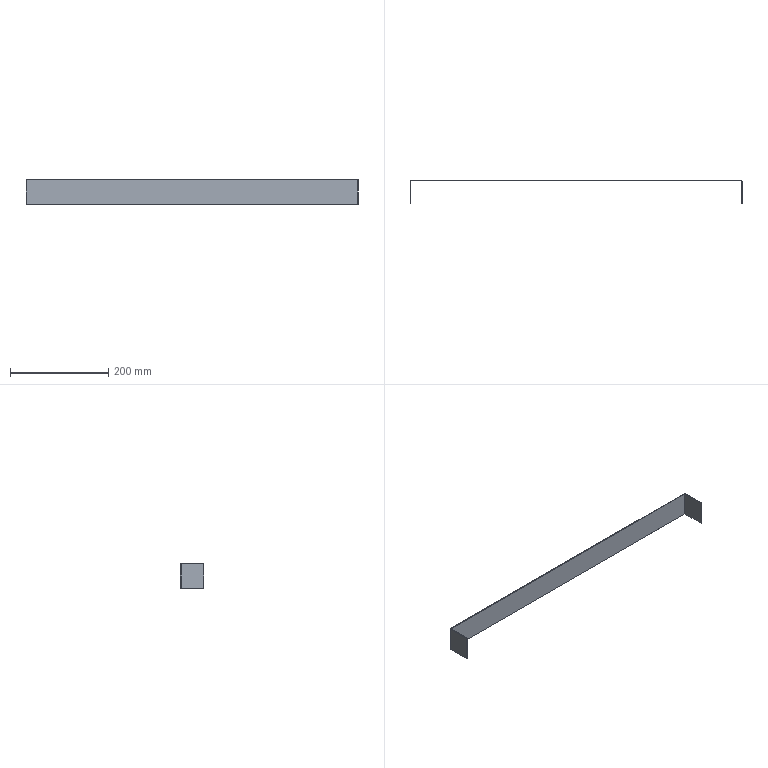Part | STEP file | C4 connector | 1 solid | 14 faces | box 677 x 48.5 x 50 mm | volume 57745 mm3 | plane 10 | cylinder 4 | commonest cylinder face diameters 1 x2 4 x2
STEP:
#1=CARTESIAN_POINT('',(0.,0.,0.));
#2=DIRECTION('',(0.,0.,1.));
#3=DIRECTION('',(1.,0.,0.));
#4=AXIS2_PLACEMENT_3D('',#1,#2,#3);
#5=CARTESIAN_POINT('',(3.5,48.5,0.));
#6=VERTEX_POINT('',#5);
#7=CARTESIAN_POINT('',(1.5,46.5,0.));
#8=VERTEX_POINT('',#7);
#9=CARTESIAN_POINT('',(3.5,46.5,0.));
#10=DIRECTION('',(0.,0.,1.));
#11=DIRECTION('',(0.,1.,0.));
#12=AXIS2_PLACEMENT_3D('',#9,#10,#11);
#13=CIRCLE('',#12,2.);
#14=CARTESIAN_POINT('',(3.5,46.5,0.));
#15=DIRECTION('',(0.,0.,1.));
#16=DIRECTION('',(0.,1.,0.));
#17=AXIS2_PLACEMENT_3D('',#14,#15,#16);
#18=CYLINDRICAL_SURFACE('',#17,2.);
#19=CARTESIAN_POINT('',(0.,0.));
#20=DIRECTION('',(1.,0.));
#21=VECTOR('',#20,1.);
#22=LINE('',#19,#21);
#23=(GEOMETRIC_REPRESENTATION_CONTEXT(2)PARAMETRIC_REPRESENTATION_CONTEXT()REPRESENTATION_CONTEXT('',''));
#24=DEFINITIONAL_REPRESENTATION('',(#22),#23);
#25=PCURVE('',#18,#24);
#26=CARTESIAN_POINT('',(340.,44.699,0.));
#27=DIRECTION('',(0.,0.,1.));
#28=DIRECTION('',(1.,0.,0.));
#29=AXIS2_PLACEMENT_3D('',#26,#27,#28);
#30=PLANE('',#29);
#31=CARTESIAN_POINT('',(-336.5,1.801));
#32=DIRECTION('',(0.,1.));
#33=AXIS2_PLACEMENT_2D('',#31,#32);
#34=CIRCLE('',#33,2.);
#35=(GEOMETRIC_REPRESENTATION_CONTEXT(2)PARAMETRIC_REPRESENTATION_CONTEXT()REPRESENTATION_CONTEXT('',''));
#36=DEFINITIONAL_REPRESENTATION('',(#34),#35);
#37=PCURVE('',#30,#36);
#38=SURFACE_CURVE('',#13,(#25,#37),.PCURVE_S1.);
#39=EDGE_CURVE('',#6,#8,#38,.T.);
#40=ORIENTED_EDGE('',*,*,#39,.T.);
#41=CARTESIAN_POINT('',(1.5,46.5,50.));
#42=VERTEX_POINT('',#41);
#43=CARTESIAN_POINT('',(1.5,46.5,0.));
#44=DIRECTION('',(0.,0.,1.));
#45=VECTOR('',#44,1.);
#46=LINE('',#43,#45);
#47=CARTESIAN_POINT('',(1.571,0.));
#48=DIRECTION('',(0.,1.));
#49=VECTOR('',#48,1.);
#50=LINE('',#47,#49);
#51=(GEOMETRIC_REPRESENTATION_CONTEXT(2)PARAMETRIC_REPRESENTATION_CONTEXT()REPRESENTATION_CONTEXT('',''));
#52=DEFINITIONAL_REPRESENTATION('',(#50),#51);
#53=PCURVE('',#18,#52);
#54=CARTESIAN_POINT('',(1.5,46.5,0.));
#55=DIRECTION('',(-1.,0.,0.));
#56=DIRECTION('',(0.,-1.,0.));
#57=AXIS2_PLACEMENT_3D('',#54,#55,#56);
#58=PLANE('',#57);
#59=CARTESIAN_POINT('',(0.,0.));
#60=DIRECTION('',(0.,1.));
#61=VECTOR('',#60,1.);
#62=LINE('',#59,#61);
#63=(GEOMETRIC_REPRESENTATION_CONTEXT(2)PARAMETRIC_REPRESENTATION_CONTEXT()REPRESENTATION_CONTEXT('',''));
#64=DEFINITIONAL_REPRESENTATION('',(#62),#63);
#65=PCURVE('',#58,#64);
#66=SURFACE_CURVE('',#46,(#53,#65),.PCURVE_S1.);
#67=EDGE_CURVE('',#8,#42,#66,.T.);
#68=ORIENTED_EDGE('',*,*,#67,.T.);
#69=CARTESIAN_POINT('',(3.5,48.5,50.));
#70=VERTEX_POINT('',#69);
#71=CARTESIAN_POINT('',(3.5,46.5,50.));
#72=DIRECTION('',(0.,0.,1.));
#73=DIRECTION('',(0.,1.,0.));
#74=AXIS2_PLACEMENT_3D('',#71,#72,#73);
#75=CIRCLE('',#74,2.);
#76=CARTESIAN_POINT('',(0.,50.));
#77=DIRECTION('',(1.,0.));
#78=VECTOR('',#77,1.);
#79=LINE('',#76,#78);
#80=(GEOMETRIC_REPRESENTATION_CONTEXT(2)PARAMETRIC_REPRESENTATION_CONTEXT()REPRESENTATION_CONTEXT('',''));
#81=DEFINITIONAL_REPRESENTATION('',(#79),#80);
#82=PCURVE('',#18,#81);
#83=CARTESIAN_POINT('',(340.,44.699,50.));
#84=DIRECTION('',(0.,0.,1.));
#85=DIRECTION('',(1.,0.,0.));
#86=AXIS2_PLACEMENT_3D('',#83,#84,#85);
#87=PLANE('',#86);
#88=CARTESIAN_POINT('',(-336.5,1.801));
#89=DIRECTION('',(0.,1.));
#90=AXIS2_PLACEMENT_2D('',#88,#89);
#91=CIRCLE('',#90,2.);
#92=(GEOMETRIC_REPRESENTATION_CONTEXT(2)PARAMETRIC_REPRESENTATION_CONTEXT()REPRESENTATION_CONTEXT('',''));
#93=DEFINITIONAL_REPRESENTATION('',(#91),#92);
#94=PCURVE('',#87,#93);
#95=SURFACE_CURVE('',#75,(#82,#94),.PCURVE_S1.);
#96=EDGE_CURVE('',#70,#42,#95,.T.);
#97=ORIENTED_EDGE('',*,*,#96,.F.);
#98=CARTESIAN_POINT('',(3.5,48.5,0.));
#99=DIRECTION('',(0.,0.,1.));
#100=VECTOR('',#99,1.);
#101=LINE('',#98,#100);
#102=CARTESIAN_POINT('',(0.,0.));
#103=DIRECTION('',(0.,1.));
#104=VECTOR('',#103,1.);
#105=LINE('',#102,#104);
#106=(GEOMETRIC_REPRESENTATION_CONTEXT(2)PARAMETRIC_REPRESENTATION_CONTEXT()REPRESENTATION_CONTEXT('',''));
#107=DEFINITIONAL_REPRESENTATION('',(#105),#106);
#108=PCURVE('',#18,#107);
#109=CARTESIAN_POINT('',(676.5,48.5,0.));
#110=DIRECTION('',(0.,1.,0.));
#111=DIRECTION('',(-1.,0.,0.));
#112=AXIS2_PLACEMENT_3D('',#109,#110,#111);
#113=PLANE('',#112);
#114=CARTESIAN_POINT('',(673.,0.));
#115=DIRECTION('',(0.,1.));
#116=VECTOR('',#115,1.);
#117=LINE('',#114,#116);
#118=(GEOMETRIC_REPRESENTATION_CONTEXT(2)PARAMETRIC_REPRESENTATION_CONTEXT()REPRESENTATION_CONTEXT('',''));
#119=DEFINITIONAL_REPRESENTATION('',(#117),#118);
#120=PCURVE('',#113,#119);
#121=SURFACE_CURVE('',#101,(#108,#120),.PCURVE_S1.);
#122=EDGE_CURVE('',#6,#70,#121,.T.);
#123=ORIENTED_EDGE('',*,*,#122,.F.);
#124=EDGE_LOOP('',(#40,#68,#97,#123));
#125=FACE_BOUND('',#124,.T.);
#126=ADVANCED_FACE('',(#125),#18,.T.);
#127=CARTESIAN_POINT('',(676.5,48.5,0.));
#128=VERTEX_POINT('',#127);
#129=CARTESIAN_POINT('',(676.5,48.5,0.));
#130=DIRECTION('',(-1.,0.,0.));
#131=VECTOR('',#130,1.);
#132=LINE('',#129,#131);
#133=CARTESIAN_POINT('',(0.,0.));
#134=DIRECTION('',(1.,0.));
#135=VECTOR('',#134,1.);
#136=LINE('',#133,#135);
#137=(GEOMETRIC_REPRESENTATION_CONTEXT(2)PARAMETRIC_REPRESENTATION_CONTEXT()REPRESENTATION_CONTEXT('',''));
#138=DEFINITIONAL_REPRESENTATION('',(#136),#137);
#139=PCURVE('',#113,#138);
#140=CARTESIAN_POINT('',(336.5,3.801));
#141=DIRECTION('',(-1.,0.));
#142=VECTOR('',#141,1.);
#143=LINE('',#140,#142);
#144=(GEOMETRIC_REPRESENTATION_CONTEXT(2)PARAMETRIC_REPRESENTATION_CONTEXT()REPRESENTATION_CONTEXT('',''));
#145=DEFINITIONAL_REPRESENTATION('',(#143),#144);
#146=PCURVE('',#30,#145);
#147=SURFACE_CURVE('',#132,(#139,#146),.PCURVE_S1.);
#148=EDGE_CURVE('',#128,#6,#147,.T.);
#149=ORIENTED_EDGE('',*,*,#148,.T.);
#150=ORIENTED_EDGE('',*,*,#122,.T.);
#151=CARTESIAN_POINT('',(676.5,48.5,50.));
#152=VERTEX_POINT('',#151);
#153=CARTESIAN_POINT('',(676.5,48.5,50.));
#154=DIRECTION('',(-1.,0.,0.));
#155=VECTOR('',#154,1.);
#156=LINE('',#153,#155);
#157=CARTESIAN_POINT('',(0.,50.));
#158=DIRECTION('',(1.,0.));
#159=VECTOR('',#158,1.);
#160=LINE('',#157,#159);
#161=(GEOMETRIC_REPRESENTATION_CONTEXT(2)PARAMETRIC_REPRESENTATION_CONTEXT()REPRESENTATION_CONTEXT('',''));
#162=DEFINITIONAL_REPRESENTATION('',(#160),#161);
#163=PCURVE('',#113,#162);
#164=CARTESIAN_POINT('',(336.5,3.801));
#165=DIRECTION('',(-1.,0.));
#166=VECTOR('',#165,1.);
#167=LINE('',#164,#166);
#168=(GEOMETRIC_REPRESENTATION_CONTEXT(2)PARAMETRIC_REPRESENTATION_CONTEXT()REPRESENTATION_CONTEXT('',''));
#169=DEFINITIONAL_REPRESENTATION('',(#167),#168);
#170=PCURVE('',#87,#169);
#171=SURFACE_CURVE('',#156,(#163,#170),.PCURVE_S1.);
#172=EDGE_CURVE('',#152,#70,#171,.T.);
#173=ORIENTED_EDGE('',*,*,#172,.F.);
#174=CARTESIAN_POINT('',(676.5,48.5,0.));
#175=DIRECTION('',(0.,0.,1.));
#176=VECTOR('',#175,1.);
#177=LINE('',#174,#176);
#178=CARTESIAN_POINT('',(0.,0.));
#179=DIRECTION('',(0.,1.));
#180=VECTOR('',#179,1.);
#181=LINE('',#178,#180);
#182=(GEOMETRIC_REPRESENTATION_CONTEXT(2)PARAMETRIC_REPRESENTATION_CONTEXT()REPRESENTATION_CONTEXT('',''));
#183=DEFINITIONAL_REPRESENTATION('',(#181),#182);
#184=PCURVE('',#113,#183);
#185=CARTESIAN_POINT('',(676.5,46.5,0.));
#186=DIRECTION('',(0.,0.,1.));
#187=DIRECTION('',(1.,0.,0.));
#188=AXIS2_PLACEMENT_3D('',#185,#186,#187);
#189=CYLINDRICAL_SURFACE('',#188,2.);
#190=CARTESIAN_POINT('',(1.571,0.));
#191=DIRECTION('',(0.,1.));
#192=VECTOR('',#191,1.);
#193=LINE('',#190,#192);
#194=(GEOMETRIC_REPRESENTATION_CONTEXT(2)PARAMETRIC_REPRESENTATION_CONTEXT()REPRESENTATION_CONTEXT('',''));
#195=DEFINITIONAL_REPRESENTATION('',(#193),#194);
#196=PCURVE('',#189,#195);
#197=SURFACE_CURVE('',#177,(#184,#196),.PCURVE_S1.);
#198=EDGE_CURVE('',#128,#152,#197,.T.);
#199=ORIENTED_EDGE('',*,*,#198,.F.);
#200=EDGE_LOOP('',(#149,#150,#173,#199));
#201=FACE_BOUND('',#200,.T.);
#202=ADVANCED_FACE('',(#201),#113,.T.);
#203=CARTESIAN_POINT('',(678.5,46.5,0.));
#204=VERTEX_POINT('',#203);
#205=CARTESIAN_POINT('',(676.5,46.5,0.));
#206=DIRECTION('',(0.,0.,1.));
#207=DIRECTION('',(1.,0.,0.));
#208=AXIS2_PLACEMENT_3D('',#205,#206,#207);
#209=CIRCLE('',#208,2.);
#210=CARTESIAN_POINT('',(0.,0.));
#211=DIRECTION('',(1.,0.));
#212=VECTOR('',#211,1.);
#213=LINE('',#210,#212);
#214=(GEOMETRIC_REPRESENTATION_CONTEXT(2)PARAMETRIC_REPRESENTATION_CONTEXT()REPRESENTATION_CONTEXT('',''));
#215=DEFINITIONAL_REPRESENTATION('',(#213),#214);
#216=PCURVE('',#189,#215);
#217=CARTESIAN_POINT('',(336.5,1.801));
#218=DIRECTION('',(1.,0.));
#219=AXIS2_PLACEMENT_2D('',#217,#218);
#220=CIRCLE('',#219,2.);
#221=(GEOMETRIC_REPRESENTATION_CONTEXT(2)PARAMETRIC_REPRESENTATION_CONTEXT()REPRESENTATION_CONTEXT('',''));
#222=DEFINITIONAL_REPRESENTATION('',(#220),#221);
#223=PCURVE('',#30,#222);
#224=SURFACE_CURVE('',#209,(#216,#223),.PCURVE_S1.);
#225=EDGE_CURVE('',#204,#128,#224,.T.);
#226=ORIENTED_EDGE('',*,*,#225,.T.);
#227=ORIENTED_EDGE('',*,*,#198,.T.);
#228=CARTESIAN_POINT('',(678.5,46.5,50.));
#229=VERTEX_POINT('',#228);
#230=CARTESIAN_POINT('',(676.5,46.5,50.));
#231=DIRECTION('',(0.,0.,1.));
#232=DIRECTION('',(1.,0.,0.));
#233=AXIS2_PLACEMENT_3D('',#230,#231,#232);
#234=CIRCLE('',#233,2.);
#235=CARTESIAN_POINT('',(0.,50.));
#236=DIRECTION('',(1.,0.));
#237=VECTOR('',#236,1.);
#238=LINE('',#235,#237);
#239=(GEOMETRIC_REPRESENTATION_CONTEXT(2)PARAMETRIC_REPRESENTATION_CONTEXT()REPRESENTATION_CONTEXT('',''));
#240=DEFINITIONAL_REPRESENTATION('',(#238),#239);
#241=PCURVE('',#189,#240);
#242=CARTESIAN_POINT('',(336.5,1.801));
#243=DIRECTION('',(1.,0.));
#244=AXIS2_PLACEMENT_2D('',#242,#243);
#245=CIRCLE('',#244,2.);
#246=(GEOMETRIC_REPRESENTATION_CONTEXT(2)PARAMETRIC_REPRESENTATION_CONTEXT()REPRESENTATION_CONTEXT('',''));
#247=DEFINITIONAL_REPRESENTATION('',(#245),#246);
#248=PCURVE('',#87,#247);
#249=SURFACE_CURVE('',#234,(#241,#248),.PCURVE_S1.);
#250=EDGE_CURVE('',#229,#152,#249,.T.);
#251=ORIENTED_EDGE('',*,*,#250,.F.);
#252=CARTESIAN_POINT('',(678.5,46.5,0.));
#253=DIRECTION('',(0.,0.,1.));
#254=VECTOR('',#253,1.);
#255=LINE('',#252,#254);
#256=CARTESIAN_POINT('',(0.,0.));
#257=DIRECTION('',(0.,1.));
#258=VECTOR('',#257,1.);
#259=LINE('',#256,#258);
#260=(GEOMETRIC_REPRESENTATION_CONTEXT(2)PARAMETRIC_REPRESENTATION_CONTEXT()REPRESENTATION_CONTEXT('',''));
#261=DEFINITIONAL_REPRESENTATION('',(#259),#260);
#262=PCURVE('',#189,#261);
#263=CARTESIAN_POINT('',(678.5,0.,0.));
#264=DIRECTION('',(1.,0.,0.));
#265=DIRECTION('',(0.,1.,0.));
#266=AXIS2_PLACEMENT_3D('',#263,#264,#265);
#267=PLANE('',#266);
#268=CARTESIAN_POINT('',(46.5,0.));
#269=DIRECTION('',(0.,1.));
#270=VECTOR('',#269,1.);
#271=LINE('',#268,#270);
#272=(GEOMETRIC_REPRESENTATION_CONTEXT(2)PARAMETRIC_REPRESENTATION_CONTEXT()REPRESENTATION_CONTEXT('',''));
#273=DEFINITIONAL_REPRESENTATION('',(#271),#272);
#274=PCURVE('',#267,#273);
#275=SURFACE_CURVE('',#255,(#262,#274),.PCURVE_S1.);
#276=EDGE_CURVE('',#204,#229,#275,.T.);
#277=ORIENTED_EDGE('',*,*,#276,.F.);
#278=EDGE_LOOP('',(#226,#227,#251,#277));
#279=FACE_BOUND('',#278,.T.);
#280=ADVANCED_FACE('',(#279),#189,.T.);
#281=CARTESIAN_POINT('',(678.5,0.,0.));
#282=VERTEX_POINT('',#281);
#283=CARTESIAN_POINT('',(678.5,0.,0.));
#284=DIRECTION('',(0.,1.,0.));
#285=VECTOR('',#284,1.);
#286=LINE('',#283,#285);
#287=CARTESIAN_POINT('',(0.,0.));
#288=DIRECTION('',(1.,0.));
#289=VECTOR('',#288,1.);
#290=LINE('',#287,#289);
#291=(GEOMETRIC_REPRESENTATION_CONTEXT(2)PARAMETRIC_REPRESENTATION_CONTEXT()REPRESENTATION_CONTEXT('',''));
#292=DEFINITIONAL_REPRESENTATION('',(#290),#291);
#293=PCURVE('',#267,#292);
#294=CARTESIAN_POINT('',(338.5,-44.699));
#295=DIRECTION('',(0.,1.));
#296=VECTOR('',#295,1.);
#297=LINE('',#294,#296);
#298=(GEOMETRIC_REPRESENTATION_CONTEXT(2)PARAMETRIC_REPRESENTATION_CONTEXT()REPRESENTATION_CONTEXT('',''));
#299=DEFINITIONAL_REPRESENTATION('',(#297),#298);
#300=PCURVE('',#30,#299);
#301=SURFACE_CURVE('',#286,(#293,#300),.PCURVE_S1.);
#302=EDGE_CURVE('',#282,#204,#301,.T.);
#303=ORIENTED_EDGE('',*,*,#302,.T.);
#304=ORIENTED_EDGE('',*,*,#276,.T.);
#305=CARTESIAN_POINT('',(678.5,0.,50.));
#306=VERTEX_POINT('',#305);
#307=CARTESIAN_POINT('',(678.5,0.,50.));
#308=DIRECTION('',(0.,1.,0.));
#309=VECTOR('',#308,1.);
#310=LINE('',#307,#309);
#311=CARTESIAN_POINT('',(0.,50.));
#312=DIRECTION('',(1.,0.));
#313=VECTOR('',#312,1.);
#314=LINE('',#311,#313);
#315=(GEOMETRIC_REPRESENTATION_CONTEXT(2)PARAMETRIC_REPRESENTATION_CONTEXT()REPRESENTATION_CONTEXT('',''));
#316=DEFINITIONAL_REPRESENTATION('',(#314),#315);
#317=PCURVE('',#267,#316);
#318=CARTESIAN_POINT('',(338.5,-44.699));
#319=DIRECTION('',(0.,1.));
#320=VECTOR('',#319,1.);
#321=LINE('',#318,#320);
#322=(GEOMETRIC_REPRESENTATION_CONTEXT(2)PARAMETRIC_REPRESENTATION_CONTEXT()REPRESENTATION_CONTEXT('',''));
#323=DEFINITIONAL_REPRESENTATION('',(#321),#322);
#324=PCURVE('',#87,#323);
#325=SURFACE_CURVE('',#310,(#317,#324),.PCURVE_S1.);
#326=EDGE_CURVE('',#306,#229,#325,.T.);
#327=ORIENTED_EDGE('',*,*,#326,.F.);
#328=CARTESIAN_POINT('',(678.5,0.,0.));
#329=DIRECTION('',(0.,0.,1.));
#330=VECTOR('',#329,1.);
#331=LINE('',#328,#330);
#332=CARTESIAN_POINT('',(0.,0.));
#333=DIRECTION('',(0.,1.));
#334=VECTOR('',#333,1.);
#335=LINE('',#332,#334);
#336=(GEOMETRIC_REPRESENTATION_CONTEXT(2)PARAMETRIC_REPRESENTATION_CONTEXT()REPRESENTATION_CONTEXT('',''));
#337=DEFINITIONAL_REPRESENTATION('',(#335),#336);
#338=PCURVE('',#267,#337);
#339=CARTESIAN_POINT('',(677.,0.,0.));
#340=DIRECTION('',(0.,-1.,0.));
#341=DIRECTION('',(1.,0.,0.));
#342=AXIS2_PLACEMENT_3D('',#339,#340,#341);
#343=PLANE('',#342);
#344=CARTESIAN_POINT('',(1.5,0.));
#345=DIRECTION('',(0.,1.));
#346=VECTOR('',#345,1.);
#347=LINE('',#344,#346);
#348=(GEOMETRIC_REPRESENTATION_CONTEXT(2)PARAMETRIC_REPRESENTATION_CONTEXT()REPRESENTATION_CONTEXT('',''));
#349=DEFINITIONAL_REPRESENTATION('',(#347),#348);
#350=PCURVE('',#343,#349);
#351=SURFACE_CURVE('',#331,(#338,#350),.PCURVE_S1.);
#352=EDGE_CURVE('',#282,#306,#351,.T.);
#353=ORIENTED_EDGE('',*,*,#352,.F.);
#354=EDGE_LOOP('',(#303,#304,#327,#353));
#355=FACE_BOUND('',#354,.T.);
#356=ADVANCED_FACE('',(#355),#267,.T.);
#357=CARTESIAN_POINT('',(677.,0.,0.));
#358=VERTEX_POINT('',#357);
#359=CARTESIAN_POINT('',(677.,0.,0.));
#360=DIRECTION('',(1.,0.,0.));
#361=VECTOR('',#360,1.);
#362=LINE('',#359,#361);
#363=CARTESIAN_POINT('',(0.,0.));
#364=DIRECTION('',(1.,0.));
#365=VECTOR('',#364,1.);
#366=LINE('',#363,#365);
#367=(GEOMETRIC_REPRESENTATION_CONTEXT(2)PARAMETRIC_REPRESENTATION_CONTEXT()REPRESENTATION_CONTEXT('',''));
#368=DEFINITIONAL_REPRESENTATION('',(#366),#367);
#369=PCURVE('',#343,#368);
#370=CARTESIAN_POINT('',(337.,-44.699));
#371=DIRECTION('',(1.,0.));
#372=VECTOR('',#371,1.);
#373=LINE('',#370,#372);
#374=(GEOMETRIC_REPRESENTATION_CONTEXT(2)PARAMETRIC_REPRESENTATION_CONTEXT()REPRESENTATION_CONTEXT('',''));
#375=DEFINITIONAL_REPRESENTATION('',(#373),#374);
#376=PCURVE('',#30,#375);
#377=SURFACE_CURVE('',#362,(#369,#376),.PCURVE_S1.);
#378=EDGE_CURVE('',#358,#282,#377,.T.);
#379=ORIENTED_EDGE('',*,*,#378,.T.);
#380=ORIENTED_EDGE('',*,*,#352,.T.);
#381=CARTESIAN_POINT('',(677.,0.,50.));
#382=VERTEX_POINT('',#381);
#383=CARTESIAN_POINT('',(677.,0.,50.));
#384=DIRECTION('',(1.,0.,0.));
#385=VECTOR('',#384,1.);
#386=LINE('',#383,#385);
#387=CARTESIAN_POINT('',(0.,50.));
#388=DIRECTION('',(1.,0.));
#389=VECTOR('',#388,1.);
#390=LINE('',#387,#389);
#391=(GEOMETRIC_REPRESENTATION_CONTEXT(2)PARAMETRIC_REPRESENTATION_CONTEXT()REPRESENTATION_CONTEXT('',''));
#392=DEFINITIONAL_REPRESENTATION('',(#390),#391);
#393=PCURVE('',#343,#392);
#394=CARTESIAN_POINT('',(337.,-44.699));
#395=DIRECTION('',(1.,0.));
#396=VECTOR('',#395,1.);
#397=LINE('',#394,#396);
#398=(GEOMETRIC_REPRESENTATION_CONTEXT(2)PARAMETRIC_REPRESENTATION_CONTEXT()REPRESENTATION_CONTEXT('',''));
#399=DEFINITIONAL_REPRESENTATION('',(#397),#398);
#400=PCURVE('',#87,#399);
#401=SURFACE_CURVE('',#386,(#393,#400),.PCURVE_S1.);
#402=EDGE_CURVE('',#382,#306,#401,.T.);
#403=ORIENTED_EDGE('',*,*,#402,.F.);
#404=CARTESIAN_POINT('',(677.,0.,0.));
#405=DIRECTION('',(0.,0.,1.));
#406=VECTOR('',#405,1.);
#407=LINE('',#404,#406);
#408=CARTESIAN_POINT('',(0.,0.));
#409=DIRECTION('',(0.,1.));
#410=VECTOR('',#409,1.);
#411=LINE('',#408,#410);
#412=(GEOMETRIC_REPRESENTATION_CONTEXT(2)PARAMETRIC_REPRESENTATION_CONTEXT()REPRESENTATION_CONTEXT('',''));
#413=DEFINITIONAL_REPRESENTATION('',(#411),#412);
#414=PCURVE('',#343,#413);
#415=CARTESIAN_POINT('',(677.,46.5,0.));
#416=DIRECTION('',(-1.,0.,0.));
#417=DIRECTION('',(0.,-1.,0.));
#418=AXIS2_PLACEMENT_3D('',#415,#416,#417);
#419=PLANE('',#418);
#420=CARTESIAN_POINT('',(46.5,0.));
#421=DIRECTION('',(0.,1.));
#422=VECTOR('',#421,1.);
#423=LINE('',#420,#422);
#424=(GEOMETRIC_REPRESENTATION_CONTEXT(2)PARAMETRIC_REPRESENTATION_CONTEXT()REPRESENTATION_CONTEXT('',''));
#425=DEFINITIONAL_REPRESENTATION('',(#423),#424);
#426=PCURVE('',#419,#425);
#427=SURFACE_CURVE('',#407,(#414,#426),.PCURVE_S1.);
#428=EDGE_CURVE('',#358,#382,#427,.T.);
#429=ORIENTED_EDGE('',*,*,#428,.F.);
#430=EDGE_LOOP('',(#379,#380,#403,#429));
#431=FACE_BOUND('',#430,.T.);
#432=ADVANCED_FACE('',(#431),#343,.T.);
#433=CARTESIAN_POINT('',(677.,46.5,0.));
#434=VERTEX_POINT('',#433);
#435=CARTESIAN_POINT('',(677.,46.5,0.));
#436=DIRECTION('',(0.,-1.,0.));
#437=VECTOR('',#436,1.);
#438=LINE('',#435,#437);
#439=CARTESIAN_POINT('',(0.,0.));
#440=DIRECTION('',(1.,0.));
#441=VECTOR('',#440,1.);
#442=LINE('',#439,#441);
#443=(GEOMETRIC_REPRESENTATION_CONTEXT(2)PARAMETRIC_REPRESENTATION_CONTEXT()REPRESENTATION_CONTEXT('',''));
#444=DEFINITIONAL_REPRESENTATION('',(#442),#443);
#445=PCURVE('',#419,#444);
#446=CARTESIAN_POINT('',(337.,1.801));
#447=DIRECTION('',(0.,-1.));
#448=VECTOR('',#447,1.);
#449=LINE('',#446,#448);
#450=(GEOMETRIC_REPRESENTATION_CONTEXT(2)PARAMETRIC_REPRESENTATION_CONTEXT()REPRESENTATION_CONTEXT('',''));
#451=DEFINITIONAL_REPRESENTATION('',(#449),#450);
#452=PCURVE('',#30,#451);
#453=SURFACE_CURVE('',#438,(#445,#452),.PCURVE_S1.);
#454=EDGE_CURVE('',#434,#358,#453,.T.);
#455=ORIENTED_EDGE('',*,*,#454,.T.);
#456=ORIENTED_EDGE('',*,*,#428,.T.);
#457=CARTESIAN_POINT('',(677.,46.5,50.));
#458=VERTEX_POINT('',#457);
#459=CARTESIAN_POINT('',(677.,46.5,50.));
#460=DIRECTION('',(0.,-1.,0.));
#461=VECTOR('',#460,1.);
#462=LINE('',#459,#461);
#463=CARTESIAN_POINT('',(0.,50.));
#464=DIRECTION('',(1.,0.));
#465=VECTOR('',#464,1.);
#466=LINE('',#463,#465);
#467=(GEOMETRIC_REPRESENTATION_CONTEXT(2)PARAMETRIC_REPRESENTATION_CONTEXT()REPRESENTATION_CONTEXT('',''));
#468=DEFINITIONAL_REPRESENTATION('',(#466),#467);
#469=PCURVE('',#419,#468);
#470=CARTESIAN_POINT('',(337.,1.801));
#471=DIRECTION('',(0.,-1.));
#472=VECTOR('',#471,1.);
#473=LINE('',#470,#472);
#474=(GEOMETRIC_REPRESENTATION_CONTEXT(2)PARAMETRIC_REPRESENTATION_CONTEXT()REPRESENTATION_CONTEXT('',''));
#475=DEFINITIONAL_REPRESENTATION('',(#473),#474);
#476=PCURVE('',#87,#475);
#477=SURFACE_CURVE('',#462,(#469,#476),.PCURVE_S1.);
#478=EDGE_CURVE('',#458,#382,#477,.T.);
#479=ORIENTED_EDGE('',*,*,#478,.F.);
#480=CARTESIAN_POINT('',(677.,46.5,0.));
#481=DIRECTION('',(0.,0.,1.));
#482=VECTOR('',#481,1.);
#483=LINE('',#480,#482);
#484=CARTESIAN_POINT('',(0.,0.));
#485=DIRECTION('',(0.,1.));
#486=VECTOR('',#485,1.);
#487=LINE('',#484,#486);
#488=(GEOMETRIC_REPRESENTATION_CONTEXT(2)PARAMETRIC_REPRESENTATION_CONTEXT()REPRESENTATION_CONTEXT('',''));
#489=DEFINITIONAL_REPRESENTATION('',(#487),#488);
#490=PCURVE('',#419,#489);
#491=CARTESIAN_POINT('',(676.5,46.5,0.));
#492=DIRECTION('',(0.,0.,1.));
#493=DIRECTION('',(-1.,0.,0.));
#494=AXIS2_PLACEMENT_3D('',#491,#492,#493);
#495=CYLINDRICAL_SURFACE('',#494,0.5);
#496=CARTESIAN_POINT('',(3.142,0.));
#497=DIRECTION('',(0.,1.));
#498=VECTOR('',#497,1.);
#499=LINE('',#496,#498);
#500=(GEOMETRIC_REPRESENTATION_CONTEXT(2)PARAMETRIC_REPRESENTATION_CONTEXT()REPRESENTATION_CONTEXT('',''));
#501=DEFINITIONAL_REPRESENTATION('',(#499),#500);
#502=PCURVE('',#495,#501);
#503=SURFACE_CURVE('',#483,(#490,#502),.PCURVE_S1.);
#504=EDGE_CURVE('',#434,#458,#503,.T.);
#505=ORIENTED_EDGE('',*,*,#504,.F.);
#506=EDGE_LOOP('',(#455,#456,#479,#505));
#507=FACE_BOUND('',#506,.T.);
#508=ADVANCED_FACE('',(#507),#419,.T.);
#509=CARTESIAN_POINT('',(676.5,47.,0.));
#510=VERTEX_POINT('',#509);
#511=CARTESIAN_POINT('',(676.5,47.,50.));
#512=VERTEX_POINT('',#511);
#513=CARTESIAN_POINT('',(676.5,47.,0.));
#514=DIRECTION('',(0.,0.,1.));
#515=VECTOR('',#514,1.);
#516=LINE('',#513,#515);
#517=CARTESIAN_POINT('',(4.712,0.));
#518=DIRECTION('',(0.,1.));
#519=VECTOR('',#518,1.);
#520=LINE('',#517,#519);
#521=(GEOMETRIC_REPRESENTATION_CONTEXT(2)PARAMETRIC_REPRESENTATION_CONTEXT()REPRESENTATION_CONTEXT('',''));
#522=DEFINITIONAL_REPRESENTATION('',(#520),#521);
#523=PCURVE('',#495,#522);
#524=CARTESIAN_POINT('',(3.5,47.,0.));
#525=DIRECTION('',(0.,-1.,0.));
#526=DIRECTION('',(1.,0.,0.));
#527=AXIS2_PLACEMENT_3D('',#524,#525,#526);
#528=PLANE('',#527);
#529=CARTESIAN_POINT('',(673.,0.));
#530=DIRECTION('',(0.,1.));
#531=VECTOR('',#530,1.);
#532=LINE('',#529,#531);
#533=(GEOMETRIC_REPRESENTATION_CONTEXT(2)PARAMETRIC_REPRESENTATION_CONTEXT()REPRESENTATION_CONTEXT('',''));
#534=DEFINITIONAL_REPRESENTATION('',(#532),#533);
#535=PCURVE('',#528,#534);
#536=SURFACE_CURVE('',#516,(#523,#535),.PCURVE_S1.);
#537=EDGE_CURVE('',#510,#512,#536,.T.);
#538=ORIENTED_EDGE('',*,*,#537,.T.);
#539=CARTESIAN_POINT('',(676.5,46.5,50.));
#540=DIRECTION('',(0.,0.,-1.));
#541=DIRECTION('',(-1.,0.,0.));
#542=AXIS2_PLACEMENT_3D('',#539,#540,#541);
#543=CIRCLE('',#542,0.5);
#544=CARTESIAN_POINT('',(6.283,50.));
#545=DIRECTION('',(-1.,0.));
#546=VECTOR('',#545,1.);
#547=LINE('',#544,#546);
#548=(GEOMETRIC_REPRESENTATION_CONTEXT(2)PARAMETRIC_REPRESENTATION_CONTEXT()REPRESENTATION_CONTEXT('',''));
#549=DEFINITIONAL_REPRESENTATION('',(#547),#548);
#550=PCURVE('',#495,#549);
#551=CARTESIAN_POINT('',(336.,1.801));
#552=CARTESIAN_POINT('',(336.,2.667));
#553=CARTESIAN_POINT('',(336.75,2.234));
#554=CARTESIAN_POINT('',(337.5,1.801));
#555=CARTESIAN_POINT('',(336.75,1.368));
#556=CARTESIAN_POINT('',(336.,0.935));
#557=CARTESIAN_POINT('',(336.,1.801));
#558=(BOUNDED_CURVE()B_SPLINE_CURVE(2,(#551,#552,#553,#554,#555,#556,#557),.UNSPECIFIED.,.T.,.F.)B_SPLINE_CURVE_WITH_KNOTS((1,2,2,2,2,1),(-2.094,0.,2.094,4.189,6.283,8.378),.UNSPECIFIED.)CURVE()GEOMETRIC_REPRESENTATION_ITEM()RATIONAL_B_SPLINE_CURVE((1.,0.5,1.,0.5,1.,0.5,1.))REPRESENTATION_ITEM(''));
#559=(GEOMETRIC_REPRESENTATION_CONTEXT(2)PARAMETRIC_REPRESENTATION_CONTEXT()REPRESENTATION_CONTEXT('',''));
#560=DEFINITIONAL_REPRESENTATION('',(#558),#559);
#561=PCURVE('',#87,#560);
#562=SURFACE_CURVE('',#543,(#550,#561),.PCURVE_S1.);
#563=EDGE_CURVE('',#512,#458,#562,.T.);
#564=ORIENTED_EDGE('',*,*,#563,.T.);
#565=ORIENTED_EDGE('',*,*,#504,.F.);
#566=CARTESIAN_POINT('',(676.5,46.5,0.));
#567=DIRECTION('',(0.,0.,-1.));
#568=DIRECTION('',(-1.,0.,0.));
#569=AXIS2_PLACEMENT_3D('',#566,#567,#568);
#570=CIRCLE('',#569,0.5);
#571=CARTESIAN_POINT('',(6.283,0.));
#572=DIRECTION('',(-1.,0.));
#573=VECTOR('',#572,1.);
#574=LINE('',#571,#573);
#575=(GEOMETRIC_REPRESENTATION_CONTEXT(2)PARAMETRIC_REPRESENTATION_CONTEXT()REPRESENTATION_CONTEXT('',''));
#576=DEFINITIONAL_REPRESENTATION('',(#574),#575);
#577=PCURVE('',#495,#576);
#578=CARTESIAN_POINT('',(336.,1.801));
#579=CARTESIAN_POINT('',(336.,2.667));
#580=CARTESIAN_POINT('',(336.75,2.234));
#581=CARTESIAN_POINT('',(337.5,1.801));
#582=CARTESIAN_POINT('',(336.75,1.368));
#583=CARTESIAN_POINT('',(336.,0.935));
#584=CARTESIAN_POINT('',(336.,1.801));
#585=(BOUNDED_CURVE()B_SPLINE_CURVE(2,(#578,#579,#580,#581,#582,#583,#584),.UNSPECIFIED.,.T.,.F.)B_SPLINE_CURVE_WITH_KNOTS((1,2,2,2,2,1),(-2.094,0.,2.094,4.189,6.283,8.378),.UNSPECIFIED.)CURVE()GEOMETRIC_REPRESENTATION_ITEM()RATIONAL_B_SPLINE_CURVE((1.,0.5,1.,0.5,1.,0.5,1.))REPRESENTATION_ITEM(''));
#586=(GEOMETRIC_REPRESENTATION_CONTEXT(2)PARAMETRIC_REPRESENTATION_CONTEXT()REPRESENTATION_CONTEXT('',''));
#587=DEFINITIONAL_REPRESENTATION('',(#585),#586);
#588=PCURVE('',#30,#587);
#589=SURFACE_CURVE('',#570,(#577,#588),.PCURVE_S1.);
#590=EDGE_CURVE('',#510,#434,#589,.T.);
#591=ORIENTED_EDGE('',*,*,#590,.F.);
#592=EDGE_LOOP('',(#538,#564,#565,#591));
#593=FACE_BOUND('',#592,.F.);
#594=ADVANCED_FACE('',(#593),#495,.F.);
#595=CARTESIAN_POINT('',(3.5,47.,0.));
#596=VERTEX_POINT('',#595);
#597=CARTESIAN_POINT('',(3.5,47.,0.));
#598=DIRECTION('',(1.,0.,0.));
#599=VECTOR('',#598,1.);
#600=LINE('',#597,#599);
#601=CARTESIAN_POINT('',(0.,0.));
#602=DIRECTION('',(1.,0.));
#603=VECTOR('',#602,1.);
#604=LINE('',#601,#603);
#605=(GEOMETRIC_REPRESENTATION_CONTEXT(2)PARAMETRIC_REPRESENTATION_CONTEXT()REPRESENTATION_CONTEXT('',''));
#606=DEFINITIONAL_REPRESENTATION('',(#604),#605);
#607=PCURVE('',#528,#606);
#608=CARTESIAN_POINT('',(-336.5,2.301));
#609=DIRECTION('',(1.,0.));
#610=VECTOR('',#609,1.);
#611=LINE('',#608,#610);
#612=(GEOMETRIC_REPRESENTATION_CONTEXT(2)PARAMETRIC_REPRESENTATION_CONTEXT()REPRESENTATION_CONTEXT('',''));
#613=DEFINITIONAL_REPRESENTATION('',(#611),#612);
#614=PCURVE('',#30,#613);
#615=SURFACE_CURVE('',#600,(#607,#614),.PCURVE_S1.);
#616=EDGE_CURVE('',#596,#510,#615,.T.);
#617=ORIENTED_EDGE('',*,*,#616,.T.);
#618=ORIENTED_EDGE('',*,*,#537,.T.);
#619=CARTESIAN_POINT('',(3.5,47.,50.));
#620=VERTEX_POINT('',#619);
#621=CARTESIAN_POINT('',(3.5,47.,50.));
#622=DIRECTION('',(1.,0.,0.));
#623=VECTOR('',#622,1.);
#624=LINE('',#621,#623);
#625=CARTESIAN_POINT('',(0.,50.));
#626=DIRECTION('',(1.,0.));
#627=VECTOR('',#626,1.);
#628=LINE('',#625,#627);
#629=(GEOMETRIC_REPRESENTATION_CONTEXT(2)PARAMETRIC_REPRESENTATION_CONTEXT()REPRESENTATION_CONTEXT('',''));
#630=DEFINITIONAL_REPRESENTATION('',(#628),#629);
#631=PCURVE('',#528,#630);
#632=CARTESIAN_POINT('',(-336.5,2.301));
#633=DIRECTION('',(1.,0.));
#634=VECTOR('',#633,1.);
#635=LINE('',#632,#634);
#636=(GEOMETRIC_REPRESENTATION_CONTEXT(2)PARAMETRIC_REPRESENTATION_CONTEXT()REPRESENTATION_CONTEXT('',''));
#637=DEFINITIONAL_REPRESENTATION('',(#635),#636);
#638=PCURVE('',#87,#637);
#639=SURFACE_CURVE('',#624,(#631,#638),.PCURVE_S1.);
#640=EDGE_CURVE('',#620,#512,#639,.T.);
#641=ORIENTED_EDGE('',*,*,#640,.F.);
#642=CARTESIAN_POINT('',(3.5,47.,0.));
#643=DIRECTION('',(0.,0.,1.));
#644=VECTOR('',#643,1.);
#645=LINE('',#642,#644);
#646=CARTESIAN_POINT('',(0.,0.));
#647=DIRECTION('',(0.,1.));
#648=VECTOR('',#647,1.);
#649=LINE('',#646,#648);
#650=(GEOMETRIC_REPRESENTATION_CONTEXT(2)PARAMETRIC_REPRESENTATION_CONTEXT()REPRESENTATION_CONTEXT('',''));
#651=DEFINITIONAL_REPRESENTATION('',(#649),#650);
#652=PCURVE('',#528,#651);
#653=CARTESIAN_POINT('',(3.5,46.5,0.));
#654=DIRECTION('',(0.,0.,1.));
#655=DIRECTION('',(0.,-1.,0.));
#656=AXIS2_PLACEMENT_3D('',#653,#654,#655);
#657=CYLINDRICAL_SURFACE('',#656,0.5);
#658=CARTESIAN_POINT('',(3.142,0.));
#659=DIRECTION('',(0.,1.));
#660=VECTOR('',#659,1.);
#661=LINE('',#658,#660);
#662=(GEOMETRIC_REPRESENTATION_CONTEXT(2)PARAMETRIC_REPRESENTATION_CONTEXT()REPRESENTATION_CONTEXT('',''));
#663=DEFINITIONAL_REPRESENTATION('',(#661),#662);
#664=PCURVE('',#657,#663);
#665=SURFACE_CURVE('',#645,(#652,#664),.PCURVE_S1.);
#666=EDGE_CURVE('',#596,#620,#665,.T.);
#667=ORIENTED_EDGE('',*,*,#666,.F.);
#668=EDGE_LOOP('',(#617,#618,#641,#667));
#669=FACE_BOUND('',#668,.T.);
#670=ADVANCED_FACE('',(#669),#528,.T.);
#671=CARTESIAN_POINT('',(3.,46.5,0.));
#672=VERTEX_POINT('',#671);
#673=CARTESIAN_POINT('',(3.,46.5,50.));
#674=VERTEX_POINT('',#673);
#675=CARTESIAN_POINT('',(3.,46.5,0.));
#676=DIRECTION('',(0.,0.,1.));
#677=VECTOR('',#676,1.);
#678=LINE('',#675,#677);
#679=CARTESIAN_POINT('',(4.712,0.));
#680=DIRECTION('',(0.,1.));
#681=VECTOR('',#680,1.);
#682=LINE('',#679,#681);
#683=(GEOMETRIC_REPRESENTATION_CONTEXT(2)PARAMETRIC_REPRESENTATION_CONTEXT()REPRESENTATION_CONTEXT('',''));
#684=DEFINITIONAL_REPRESENTATION('',(#682),#683);
#685=PCURVE('',#657,#684);
#686=CARTESIAN_POINT('',(3.,0.,0.));
#687=DIRECTION('',(1.,0.,0.));
#688=DIRECTION('',(0.,1.,0.));
#689=AXIS2_PLACEMENT_3D('',#686,#687,#688);
#690=PLANE('',#689);
#691=CARTESIAN_POINT('',(46.5,0.));
#692=DIRECTION('',(0.,1.));
#693=VECTOR('',#692,1.);
#694=LINE('',#691,#693);
#695=(GEOMETRIC_REPRESENTATION_CONTEXT(2)PARAMETRIC_REPRESENTATION_CONTEXT()REPRESENTATION_CONTEXT('',''));
#696=DEFINITIONAL_REPRESENTATION('',(#694),#695);
#697=PCURVE('',#690,#696);
#698=SURFACE_CURVE('',#678,(#685,#697),.PCURVE_S1.);
#699=EDGE_CURVE('',#672,#674,#698,.T.);
#700=ORIENTED_EDGE('',*,*,#699,.T.);
#701=CARTESIAN_POINT('',(3.5,46.5,50.));
#702=DIRECTION('',(0.,0.,-1.));
#703=DIRECTION('',(0.,-1.,0.));
#704=AXIS2_PLACEMENT_3D('',#701,#702,#703);
#705=CIRCLE('',#704,0.5);
#706=CARTESIAN_POINT('',(6.283,50.));
#707=DIRECTION('',(-1.,0.));
#708=VECTOR('',#707,1.);
#709=LINE('',#706,#708);
#710=(GEOMETRIC_REPRESENTATION_CONTEXT(2)PARAMETRIC_REPRESENTATION_CONTEXT()REPRESENTATION_CONTEXT('',''));
#711=DEFINITIONAL_REPRESENTATION('',(#709),#710);
#712=PCURVE('',#657,#711);
#713=CARTESIAN_POINT('',(-336.5,1.301));
#714=CARTESIAN_POINT('',(-337.366,1.301));
#715=CARTESIAN_POINT('',(-336.933,2.051));
#716=CARTESIAN_POINT('',(-336.5,2.801));
#717=CARTESIAN_POINT('',(-336.067,2.051));
#718=CARTESIAN_POINT('',(-335.634,1.301));
#719=CARTESIAN_POINT('',(-336.5,1.301));
#720=(BOUNDED_CURVE()B_SPLINE_CURVE(2,(#713,#714,#715,#716,#717,#718,#719),.UNSPECIFIED.,.T.,.F.)B_SPLINE_CURVE_WITH_KNOTS((1,2,2,2,2,1),(-2.094,0.,2.094,4.189,6.283,8.378),.UNSPECIFIED.)CURVE()GEOMETRIC_REPRESENTATION_ITEM()RATIONAL_B_SPLINE_CURVE((1.,0.5,1.,0.5,1.,0.5,1.))REPRESENTATION_ITEM(''));
#721=(GEOMETRIC_REPRESENTATION_CONTEXT(2)PARAMETRIC_REPRESENTATION_CONTEXT()REPRESENTATION_CONTEXT('',''));
#722=DEFINITIONAL_REPRESENTATION('',(#720),#721);
#723=PCURVE('',#87,#722);
#724=SURFACE_CURVE('',#705,(#712,#723),.PCURVE_S1.);
#725=EDGE_CURVE('',#674,#620,#724,.T.);
#726=ORIENTED_EDGE('',*,*,#725,.T.);
#727=ORIENTED_EDGE('',*,*,#666,.F.);
#728=CARTESIAN_POINT('',(3.5,46.5,0.));
#729=DIRECTION('',(0.,0.,-1.));
#730=DIRECTION('',(0.,-1.,0.));
#731=AXIS2_PLACEMENT_3D('',#728,#729,#730);
#732=CIRCLE('',#731,0.5);
#733=CARTESIAN_POINT('',(6.283,0.));
#734=DIRECTION('',(-1.,0.));
#735=VECTOR('',#734,1.);
#736=LINE('',#733,#735);
#737=(GEOMETRIC_REPRESENTATION_CONTEXT(2)PARAMETRIC_REPRESENTATION_CONTEXT()REPRESENTATION_CONTEXT('',''));
#738=DEFINITIONAL_REPRESENTATION('',(#736),#737);
#739=PCURVE('',#657,#738);
#740=CARTESIAN_POINT('',(-336.5,1.301));
#741=CARTESIAN_POINT('',(-337.366,1.301));
#742=CARTESIAN_POINT('',(-336.933,2.051));
#743=CARTESIAN_POINT('',(-336.5,2.801));
#744=CARTESIAN_POINT('',(-336.067,2.051));
#745=CARTESIAN_POINT('',(-335.634,1.301));
#746=CARTESIAN_POINT('',(-336.5,1.301));
#747=(BOUNDED_CURVE()B_SPLINE_CURVE(2,(#740,#741,#742,#743,#744,#745,#746),.UNSPECIFIED.,.T.,.F.)B_SPLINE_CURVE_WITH_KNOTS((1,2,2,2,2,1),(-2.094,0.,2.094,4.189,6.283,8.378),.UNSPECIFIED.)CURVE()GEOMETRIC_REPRESENTATION_ITEM()RATIONAL_B_SPLINE_CURVE((1.,0.5,1.,0.5,1.,0.5,1.))REPRESENTATION_ITEM(''));
#748=(GEOMETRIC_REPRESENTATION_CONTEXT(2)PARAMETRIC_REPRESENTATION_CONTEXT()REPRESENTATION_CONTEXT('',''));
#749=DEFINITIONAL_REPRESENTATION('',(#747),#748);
#750=PCURVE('',#30,#749);
#751=SURFACE_CURVE('',#732,(#739,#750),.PCURVE_S1.);
#752=EDGE_CURVE('',#672,#596,#751,.T.);
#753=ORIENTED_EDGE('',*,*,#752,.F.);
#754=EDGE_LOOP('',(#700,#726,#727,#753));
#755=FACE_BOUND('',#754,.F.);
#756=ADVANCED_FACE('',(#755),#657,.F.);
#757=CARTESIAN_POINT('',(3.,0.,0.));
#758=VERTEX_POINT('',#757);
#759=CARTESIAN_POINT('',(3.,0.,0.));
#760=DIRECTION('',(0.,1.,0.));
#761=VECTOR('',#760,1.);
#762=LINE('',#759,#761);
#763=CARTESIAN_POINT('',(0.,0.));
#764=DIRECTION('',(1.,0.));
#765=VECTOR('',#764,1.);
#766=LINE('',#763,#765);
#767=(GEOMETRIC_REPRESENTATION_CONTEXT(2)PARAMETRIC_REPRESENTATION_CONTEXT()REPRESENTATION_CONTEXT('',''));
#768=DEFINITIONAL_REPRESENTATION('',(#766),#767);
#769=PCURVE('',#690,#768);
#770=CARTESIAN_POINT('',(-337.,-44.699));
#771=DIRECTION('',(0.,1.));
#772=VECTOR('',#771,1.);
#773=LINE('',#770,#772);
#774=(GEOMETRIC_REPRESENTATION_CONTEXT(2)PARAMETRIC_REPRESENTATION_CONTEXT()REPRESENTATION_CONTEXT('',''));
#775=DEFINITIONAL_REPRESENTATION('',(#773),#774);
#776=PCURVE('',#30,#775);
#777=SURFACE_CURVE('',#762,(#769,#776),.PCURVE_S1.);
#778=EDGE_CURVE('',#758,#672,#777,.T.);
#779=ORIENTED_EDGE('',*,*,#778,.T.);
#780=ORIENTED_EDGE('',*,*,#699,.T.);
#781=CARTESIAN_POINT('',(3.,0.,50.));
#782=VERTEX_POINT('',#781);
#783=CARTESIAN_POINT('',(3.,0.,50.));
#784=DIRECTION('',(0.,1.,0.));
#785=VECTOR('',#784,1.);
#786=LINE('',#783,#785);
#787=CARTESIAN_POINT('',(0.,50.));
#788=DIRECTION('',(1.,0.));
#789=VECTOR('',#788,1.);
#790=LINE('',#787,#789);
#791=(GEOMETRIC_REPRESENTATION_CONTEXT(2)PARAMETRIC_REPRESENTATION_CONTEXT()REPRESENTATION_CONTEXT('',''));
#792=DEFINITIONAL_REPRESENTATION('',(#790),#791);
#793=PCURVE('',#690,#792);
#794=CARTESIAN_POINT('',(-337.,-44.699));
#795=DIRECTION('',(0.,1.));
#796=VECTOR('',#795,1.);
#797=LINE('',#794,#796);
#798=(GEOMETRIC_REPRESENTATION_CONTEXT(2)PARAMETRIC_REPRESENTATION_CONTEXT()REPRESENTATION_CONTEXT('',''));
#799=DEFINITIONAL_REPRESENTATION('',(#797),#798);
#800=PCURVE('',#87,#799);
#801=SURFACE_CURVE('',#786,(#793,#800),.PCURVE_S1.);
#802=EDGE_CURVE('',#782,#674,#801,.T.);
#803=ORIENTED_EDGE('',*,*,#802,.F.);
#804=CARTESIAN_POINT('',(3.,0.,0.));
#805=DIRECTION('',(0.,0.,1.));
#806=VECTOR('',#805,1.);
#807=LINE('',#804,#806);
#808=CARTESIAN_POINT('',(0.,0.));
#809=DIRECTION('',(0.,1.));
#810=VECTOR('',#809,1.);
#811=LINE('',#808,#810);
#812=(GEOMETRIC_REPRESENTATION_CONTEXT(2)PARAMETRIC_REPRESENTATION_CONTEXT()REPRESENTATION_CONTEXT('',''));
#813=DEFINITIONAL_REPRESENTATION('',(#811),#812);
#814=PCURVE('',#690,#813);
#815=CARTESIAN_POINT('',(1.5,0.,0.));
#816=DIRECTION('',(0.,-1.,0.));
#817=DIRECTION('',(1.,0.,0.));
#818=AXIS2_PLACEMENT_3D('',#815,#816,#817);
#819=PLANE('',#818);
#820=CARTESIAN_POINT('',(1.5,0.));
#821=DIRECTION('',(0.,1.));
#822=VECTOR('',#821,1.);
#823=LINE('',#820,#822);
#824=(GEOMETRIC_REPRESENTATION_CONTEXT(2)PARAMETRIC_REPRESENTATION_CONTEXT()REPRESENTATION_CONTEXT('',''));
#825=DEFINITIONAL_REPRESENTATION('',(#823),#824);
#826=PCURVE('',#819,#825);
#827=SURFACE_CURVE('',#807,(#814,#826),.PCURVE_S1.);
#828=EDGE_CURVE('',#758,#782,#827,.T.);
#829=ORIENTED_EDGE('',*,*,#828,.F.);
#830=EDGE_LOOP('',(#779,#780,#803,#829));
#831=FACE_BOUND('',#830,.T.);
#832=ADVANCED_FACE('',(#831),#690,.T.);
#833=CARTESIAN_POINT('',(1.5,0.,0.));
#834=VERTEX_POINT('',#833);
#835=CARTESIAN_POINT('',(1.5,0.,0.));
#836=DIRECTION('',(1.,0.,0.));
#837=VECTOR('',#836,1.);
#838=LINE('',#835,#837);
#839=CARTESIAN_POINT('',(0.,0.));
#840=DIRECTION('',(1.,0.));
#841=VECTOR('',#840,1.);
#842=LINE('',#839,#841);
#843=(GEOMETRIC_REPRESENTATION_CONTEXT(2)PARAMETRIC_REPRESENTATION_CONTEXT()REPRESENTATION_CONTEXT('',''));
#844=DEFINITIONAL_REPRESENTATION('',(#842),#843);
#845=PCURVE('',#819,#844);
#846=CARTESIAN_POINT('',(-338.5,-44.699));
#847=DIRECTION('',(1.,0.));
#848=VECTOR('',#847,1.);
#849=LINE('',#846,#848);
#850=(GEOMETRIC_REPRESENTATION_CONTEXT(2)PARAMETRIC_REPRESENTATION_CONTEXT()REPRESENTATION_CONTEXT('',''));
#851=DEFINITIONAL_REPRESENTATION('',(#849),#850);
#852=PCURVE('',#30,#851);
#853=SURFACE_CURVE('',#838,(#845,#852),.PCURVE_S1.);
#854=EDGE_CURVE('',#834,#758,#853,.T.);
#855=ORIENTED_EDGE('',*,*,#854,.T.);
#856=ORIENTED_EDGE('',*,*,#828,.T.);
#857=CARTESIAN_POINT('',(1.5,0.,50.));
#858=VERTEX_POINT('',#857);
#859=CARTESIAN_POINT('',(1.5,0.,50.));
#860=DIRECTION('',(1.,0.,0.));
#861=VECTOR('',#860,1.);
#862=LINE('',#859,#861);
#863=CARTESIAN_POINT('',(0.,50.));
#864=DIRECTION('',(1.,0.));
#865=VECTOR('',#864,1.);
#866=LINE('',#863,#865);
#867=(GEOMETRIC_REPRESENTATION_CONTEXT(2)PARAMETRIC_REPRESENTATION_CONTEXT()REPRESENTATION_CONTEXT('',''));
#868=DEFINITIONAL_REPRESENTATION('',(#866),#867);
#869=PCURVE('',#819,#868);
#870=CARTESIAN_POINT('',(-338.5,-44.699));
#871=DIRECTION('',(1.,0.));
#872=VECTOR('',#871,1.);
#873=LINE('',#870,#872);
#874=(GEOMETRIC_REPRESENTATION_CONTEXT(2)PARAMETRIC_REPRESENTATION_CONTEXT()REPRESENTATION_CONTEXT('',''));
#875=DEFINITIONAL_REPRESENTATION('',(#873),#874);
#876=PCURVE('',#87,#875);
#877=SURFACE_CURVE('',#862,(#869,#876),.PCURVE_S1.);
#878=EDGE_CURVE('',#858,#782,#877,.T.);
#879=ORIENTED_EDGE('',*,*,#878,.F.);
#880=CARTESIAN_POINT('',(1.5,0.,0.));
#881=DIRECTION('',(0.,0.,1.));
#882=VECTOR('',#881,1.);
#883=LINE('',#880,#882);
#884=CARTESIAN_POINT('',(0.,0.));
#885=DIRECTION('',(0.,1.));
#886=VECTOR('',#885,1.);
#887=LINE('',#884,#886);
#888=(GEOMETRIC_REPRESENTATION_CONTEXT(2)PARAMETRIC_REPRESENTATION_CONTEXT()REPRESENTATION_CONTEXT('',''));
#889=DEFINITIONAL_REPRESENTATION('',(#887),#888);
#890=PCURVE('',#819,#889);
#891=CARTESIAN_POINT('',(46.5,0.));
#892=DIRECTION('',(0.,1.));
#893=VECTOR('',#892,1.);
#894=LINE('',#891,#893);
#895=(GEOMETRIC_REPRESENTATION_CONTEXT(2)PARAMETRIC_REPRESENTATION_CONTEXT()REPRESENTATION_CONTEXT('',''));
#896=DEFINITIONAL_REPRESENTATION('',(#894),#895);
#897=PCURVE('',#58,#896);
#898=SURFACE_CURVE('',#883,(#890,#897),.PCURVE_S1.);
#899=EDGE_CURVE('',#834,#858,#898,.T.);
#900=ORIENTED_EDGE('',*,*,#899,.F.);
#901=EDGE_LOOP('',(#855,#856,#879,#900));
#902=FACE_BOUND('',#901,.T.);
#903=ADVANCED_FACE('',(#902),#819,.T.);
#904=CARTESIAN_POINT('',(1.5,46.5,0.));
#905=DIRECTION('',(0.,-1.,0.));
#906=VECTOR('',#905,1.);
#907=LINE('',#904,#906);
#908=CARTESIAN_POINT('',(0.,0.));
#909=DIRECTION('',(1.,0.));
#910=VECTOR('',#909,1.);
#911=LINE('',#908,#910);
#912=(GEOMETRIC_REPRESENTATION_CONTEXT(2)PARAMETRIC_REPRESENTATION_CONTEXT()REPRESENTATION_CONTEXT('',''));
#913=DEFINITIONAL_REPRESENTATION('',(#911),#912);
#914=PCURVE('',#58,#913);
#915=CARTESIAN_POINT('',(-338.5,1.801));
#916=DIRECTION('',(0.,-1.));
#917=VECTOR('',#916,1.);
#918=LINE('',#915,#917);
#919=(GEOMETRIC_REPRESENTATION_CONTEXT(2)PARAMETRIC_REPRESENTATION_CONTEXT()REPRESENTATION_CONTEXT('',''));
#920=DEFINITIONAL_REPRESENTATION('',(#918),#919);
#921=PCURVE('',#30,#920);
#922=SURFACE_CURVE('',#907,(#914,#921),.PCURVE_S1.);
#923=EDGE_CURVE('',#8,#834,#922,.T.);
#924=ORIENTED_EDGE('',*,*,#923,.T.);
#925=ORIENTED_EDGE('',*,*,#899,.T.);
#926=CARTESIAN_POINT('',(1.5,46.5,50.));
#927=DIRECTION('',(0.,-1.,0.));
#928=VECTOR('',#927,1.);
#929=LINE('',#926,#928);
#930=CARTESIAN_POINT('',(0.,50.));
#931=DIRECTION('',(1.,0.));
#932=VECTOR('',#931,1.);
#933=LINE('',#930,#932);
#934=(GEOMETRIC_REPRESENTATION_CONTEXT(2)PARAMETRIC_REPRESENTATION_CONTEXT()REPRESENTATION_CONTEXT('',''));
#935=DEFINITIONAL_REPRESENTATION('',(#933),#934);
#936=PCURVE('',#58,#935);
#937=CARTESIAN_POINT('',(-338.5,1.801));
#938=DIRECTION('',(0.,-1.));
#939=VECTOR('',#938,1.);
#940=LINE('',#937,#939);
#941=(GEOMETRIC_REPRESENTATION_CONTEXT(2)PARAMETRIC_REPRESENTATION_CONTEXT()REPRESENTATION_CONTEXT('',''));
#942=DEFINITIONAL_REPRESENTATION('',(#940),#941);
#943=PCURVE('',#87,#942);
#944=SURFACE_CURVE('',#929,(#936,#943),.PCURVE_S1.);
#945=EDGE_CURVE('',#42,#858,#944,.T.);
#946=ORIENTED_EDGE('',*,*,#945,.F.);
#947=ORIENTED_EDGE('',*,*,#67,.F.);
#948=EDGE_LOOP('',(#924,#925,#946,#947));
#949=FACE_BOUND('',#948,.T.);
#950=ADVANCED_FACE('',(#949),#58,.T.);
#951=ORIENTED_EDGE('',*,*,#945,.T.);
#952=ORIENTED_EDGE('',*,*,#878,.T.);
#953=ORIENTED_EDGE('',*,*,#802,.T.);
#954=ORIENTED_EDGE('',*,*,#725,.T.);
#955=ORIENTED_EDGE('',*,*,#640,.T.);
#956=ORIENTED_EDGE('',*,*,#563,.T.);
#957=ORIENTED_EDGE('',*,*,#478,.T.);
#958=ORIENTED_EDGE('',*,*,#402,.T.);
#959=ORIENTED_EDGE('',*,*,#326,.T.);
#960=ORIENTED_EDGE('',*,*,#250,.T.);
#961=ORIENTED_EDGE('',*,*,#172,.T.);
#962=ORIENTED_EDGE('',*,*,#96,.T.);
#963=EDGE_LOOP('',(#951,#952,#953,#954,#955,#956,#957,#958,#959,#960,#961,#962));
#964=FACE_BOUND('',#963,.T.);
#965=ADVANCED_FACE('',(#964),#87,.T.);
#966=ORIENTED_EDGE('',*,*,#923,.F.);
#967=ORIENTED_EDGE('',*,*,#39,.F.);
#968=ORIENTED_EDGE('',*,*,#148,.F.);
#969=ORIENTED_EDGE('',*,*,#225,.F.);
#970=ORIENTED_EDGE('',*,*,#302,.F.);
#971=ORIENTED_EDGE('',*,*,#378,.F.);
#972=ORIENTED_EDGE('',*,*,#454,.F.);
#973=ORIENTED_EDGE('',*,*,#590,.F.);
#974=ORIENTED_EDGE('',*,*,#616,.F.);
#975=ORIENTED_EDGE('',*,*,#752,.F.);
#976=ORIENTED_EDGE('',*,*,#778,.F.);
#977=ORIENTED_EDGE('',*,*,#854,.F.);
#978=EDGE_LOOP('',(#966,#967,#968,#969,#970,#971,#972,#973,#974,#975,#976,#977));
#979=FACE_BOUND('',#978,.T.);
#980=ADVANCED_FACE('',(#979),#30,.F.);
#981=CLOSED_SHELL('',(#126,#202,#280,#356,#432,#508,#594,#670,#756,#832,#903,#950,#965,#980));
#982=MANIFOLD_SOLID_BREP('',#981);
#983=(LENGTH_UNIT()NAMED_UNIT(*)SI_UNIT(.MILLI.,.METRE.));
#984=UNCERTAINTY_MEASURE_WITH_UNIT(LENGTH_MEASURE(0.0000001),#983,'','');
#985=(NAMED_UNIT(*)PLANE_ANGLE_UNIT()SI_UNIT($,.RADIAN.));
#986=(NAMED_UNIT(*)SI_UNIT($,.STERADIAN.)SOLID_ANGLE_UNIT());
#987=(GEOMETRIC_REPRESENTATION_CONTEXT(3)GLOBAL_UNCERTAINTY_ASSIGNED_CONTEXT((#984))GLOBAL_UNIT_ASSIGNED_CONTEXT((#983,#985,#986))REPRESENTATION_CONTEXT('',''));
#988=ADVANCED_BREP_SHAPE_REPRESENTATION('',(#4,#982),#987);